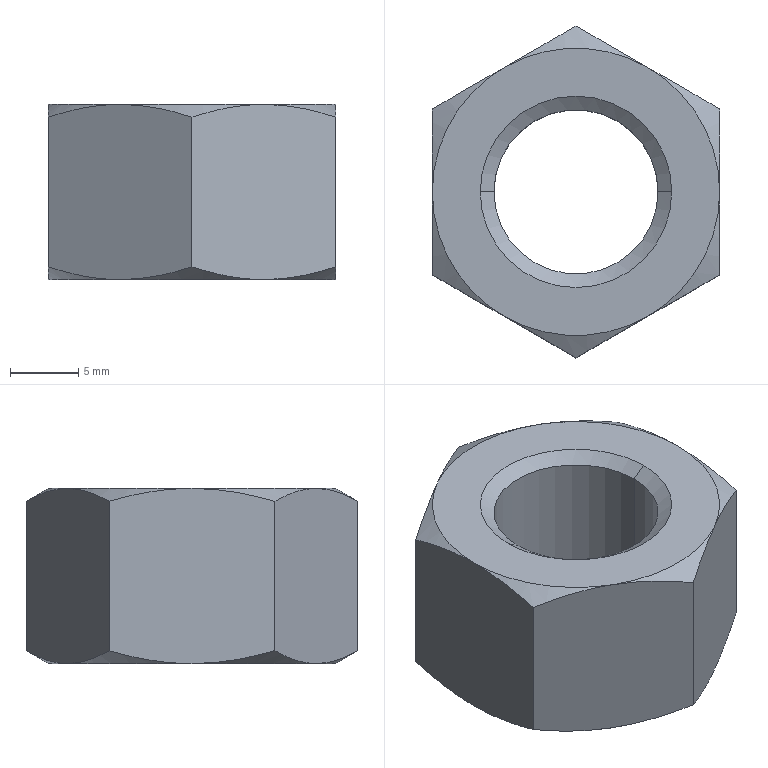Part | STEP file | hex nut style 1_am_B18.2.4.1M - Hex nut, Style 1,  M14 x 2 --D-N | 1 solid | 28 faces | box 21 x 24.249 x 12.8 mm | volume 3392 mm3 | cone 16 | plane 8 | cylinder 4 | commonest cylinder face diameters 12 x2 14 x2